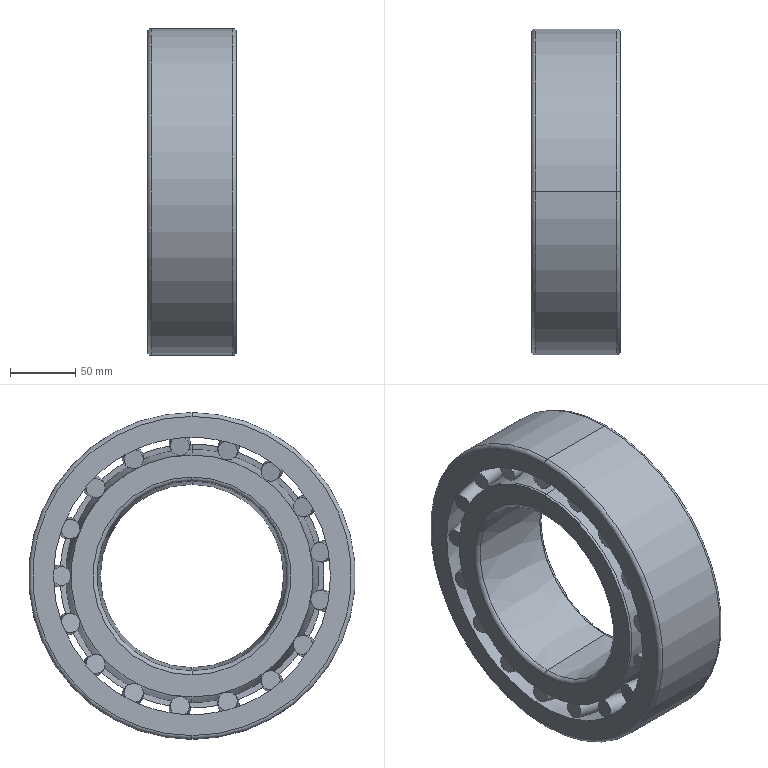Part | SolidWorks | features Revolution 3, CirPattern 1, Fillet 1, MirrorPattern 1 | 1 solid | 202 faces | box 68 x 250 x 250 mm | volume 1755852 mm3 | torus 86 | plane 72 | cone 38 | cylinder 4 | sphere 2 | commonest cylinder face diameters 201.875 x2 250 x2